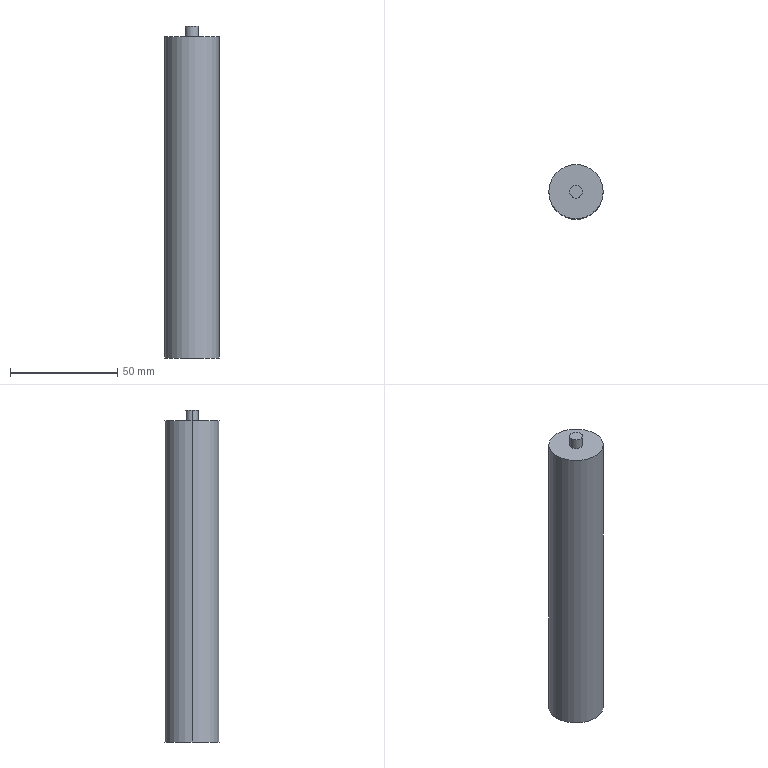Part | SolidWorks | features BaseBody 1 | 1 solid | 10 faces | box 25.4 x 25.4 x 155 mm | volume 75865 mm3 | cylinder 6 | plane 4 | commonest cylinder face diameters 6 x4 25.4 x2
STEP:
#1=CARTESIAN_POINT('',(12.7,0.,-150.));
#2=VERTEX_POINT('',#1);
#3=CARTESIAN_POINT('',(-12.7,0.,-150.));
#4=VERTEX_POINT('',#3);
#5=CARTESIAN_POINT('',(0.,0.,-150.));
#6=DIRECTION('',(0.,0.,1.));
#7=DIRECTION('',(1.,0.,0.));
#8=AXIS2_PLACEMENT_3D('',#5,#6,#7);
#9=CIRCLE('',#8,12.7);
#10=EDGE_CURVE('',#2,#4,#9,.T.);
#11=ORIENTED_EDGE('',*,*,#10,.T.);
#12=CARTESIAN_POINT('',(-12.7,0.,0.));
#13=VERTEX_POINT('',#12);
#14=CARTESIAN_POINT('',(-12.7,0.,-150.));
#15=DIRECTION('',(0.,0.,1.));
#16=VECTOR('',#15,1000.);
#17=LINE('',#14,#16);
#18=EDGE_CURVE('',#4,#13,#17,.T.);
#19=ORIENTED_EDGE('',*,*,#18,.T.);
#20=CARTESIAN_POINT('',(12.7,0.,0.));
#21=VERTEX_POINT('',#20);
#22=CARTESIAN_POINT('',(0.,0.,0.));
#23=DIRECTION('',(0.,0.,-1.));
#24=DIRECTION('',(1.,0.,0.));
#25=AXIS2_PLACEMENT_3D('',#22,#23,#24);
#26=CIRCLE('',#25,12.7);
#27=EDGE_CURVE('',#13,#21,#26,.T.);
#28=ORIENTED_EDGE('',*,*,#27,.T.);
#29=CARTESIAN_POINT('',(12.7,0.,-150.));
#30=DIRECTION('',(0.,0.,1.));
#31=VECTOR('',#30,1000.);
#32=LINE('',#29,#31);
#33=EDGE_CURVE('',#2,#21,#32,.T.);
#34=ORIENTED_EDGE('',*,*,#33,.F.);
#35=EDGE_LOOP('',(#11,#19,#28,#34));
#36=FACE_OUTER_BOUND('',#35,.T.);
#37=CARTESIAN_POINT('',(0.,0.,-150.));
#38=DIRECTION('',(0.,0.,1.));
#39=DIRECTION('',(1.,0.,0.));
#40=AXIS2_PLACEMENT_3D('',#37,#38,#39);
#41=CYLINDRICAL_SURFACE('',#40,12.7);
#42=ADVANCED_FACE('',(#36),#41,.T.);
#43=CARTESIAN_POINT('',(-3.,0.,5.));
#44=VERTEX_POINT('',#43);
#45=CARTESIAN_POINT('',(3.,0.,5.));
#46=VERTEX_POINT('',#45);
#47=CARTESIAN_POINT('',(0.,0.,5.));
#48=DIRECTION('',(0.,0.,-1.));
#49=DIRECTION('',(-1.,0.,0.));
#50=AXIS2_PLACEMENT_3D('',#47,#48,#49);
#51=CIRCLE('',#50,3.);
#52=EDGE_CURVE('',#44,#46,#51,.T.);
#53=ORIENTED_EDGE('',*,*,#52,.T.);
#54=CARTESIAN_POINT('',(3.,0.,0.));
#55=VERTEX_POINT('',#54);
#56=CARTESIAN_POINT('',(3.,0.,5.));
#57=DIRECTION('',(0.,0.,-1.));
#58=VECTOR('',#57,1000.);
#59=LINE('',#56,#58);
#60=EDGE_CURVE('',#46,#55,#59,.T.);
#61=ORIENTED_EDGE('',*,*,#60,.T.);
#62=CARTESIAN_POINT('',(-3.,0.,0.));
#63=VERTEX_POINT('',#62);
#64=CARTESIAN_POINT('',(0.,0.,0.));
#65=DIRECTION('',(0.,0.,-1.));
#66=DIRECTION('',(-1.,0.,0.));
#67=AXIS2_PLACEMENT_3D('',#64,#65,#66);
#68=CIRCLE('',#67,3.);
#69=EDGE_CURVE('',#63,#55,#68,.T.);
#70=ORIENTED_EDGE('',*,*,#69,.F.);
#71=CARTESIAN_POINT('',(-3.,0.,5.));
#72=DIRECTION('',(0.,0.,-1.));
#73=VECTOR('',#72,1000.);
#74=LINE('',#71,#73);
#75=EDGE_CURVE('',#44,#63,#74,.T.);
#76=ORIENTED_EDGE('',*,*,#75,.F.);
#77=EDGE_LOOP('',(#53,#61,#70,#76));
#78=FACE_OUTER_BOUND('',#77,.T.);
#79=CARTESIAN_POINT('',(0.,0.,5.));
#80=DIRECTION('',(0.,0.,-1.));
#81=DIRECTION('',(-1.,0.,0.));
#82=AXIS2_PLACEMENT_3D('',#79,#80,#81);
#83=CYLINDRICAL_SURFACE('',#82,3.);
#84=ADVANCED_FACE('',(#78),#83,.T.);
#85=CARTESIAN_POINT('',(3.,0.,-140.));
#86=VERTEX_POINT('',#85);
#87=CARTESIAN_POINT('',(-3.,0.,-140.));
#88=VERTEX_POINT('',#87);
#89=CARTESIAN_POINT('',(0.,0.,-140.));
#90=DIRECTION('',(0.,0.,-1.));
#91=DIRECTION('',(-1.,0.,0.));
#92=AXIS2_PLACEMENT_3D('',#89,#90,#91);
#93=CIRCLE('',#92,3.);
#94=EDGE_CURVE('',#86,#88,#93,.T.);
#95=ORIENTED_EDGE('',*,*,#94,.F.);
#96=CARTESIAN_POINT('',(3.,0.,-150.));
#97=VERTEX_POINT('',#96);
#98=CARTESIAN_POINT('',(3.,0.,-140.));
#99=DIRECTION('',(0.,0.,-1.));
#100=VECTOR('',#99,1000.);
#101=LINE('',#98,#100);
#102=EDGE_CURVE('',#86,#97,#101,.T.);
#103=ORIENTED_EDGE('',*,*,#102,.T.);
#104=CARTESIAN_POINT('',(-3.,0.,-150.));
#105=VERTEX_POINT('',#104);
#106=CARTESIAN_POINT('',(0.,0.,-150.));
#107=DIRECTION('',(0.,0.,-1.));
#108=DIRECTION('',(-1.,0.,0.));
#109=AXIS2_PLACEMENT_3D('',#106,#107,#108);
#110=CIRCLE('',#109,3.);
#111=EDGE_CURVE('',#97,#105,#110,.T.);
#112=ORIENTED_EDGE('',*,*,#111,.T.);
#113=CARTESIAN_POINT('',(-3.,0.,-140.));
#114=DIRECTION('',(0.,0.,-1.));
#115=VECTOR('',#114,1000.);
#116=LINE('',#113,#115);
#117=EDGE_CURVE('',#88,#105,#116,.T.);
#118=ORIENTED_EDGE('',*,*,#117,.F.);
#119=EDGE_LOOP('',(#95,#103,#112,#118));
#120=FACE_OUTER_BOUND('',#119,.T.);
#121=CARTESIAN_POINT('',(0.,0.,-140.));
#122=DIRECTION('',(0.,0.,-1.));
#123=DIRECTION('',(-1.,0.,0.));
#124=AXIS2_PLACEMENT_3D('',#121,#122,#123);
#125=CYLINDRICAL_SURFACE('',#124,3.);
#126=ADVANCED_FACE('',(#120),#125,.F.);
#127=ORIENTED_EDGE('',*,*,#18,.F.);
#128=CARTESIAN_POINT('',(0.,0.,-150.));
#129=DIRECTION('',(0.,0.,1.));
#130=DIRECTION('',(1.,0.,0.));
#131=AXIS2_PLACEMENT_3D('',#128,#129,#130);
#132=CIRCLE('',#131,12.7);
#133=EDGE_CURVE('',#4,#2,#132,.T.);
#134=ORIENTED_EDGE('',*,*,#133,.T.);
#135=ORIENTED_EDGE('',*,*,#33,.T.);
#136=CARTESIAN_POINT('',(0.,0.,0.));
#137=DIRECTION('',(0.,0.,-1.));
#138=DIRECTION('',(1.,0.,0.));
#139=AXIS2_PLACEMENT_3D('',#136,#137,#138);
#140=CIRCLE('',#139,12.7);
#141=EDGE_CURVE('',#21,#13,#140,.T.);
#142=ORIENTED_EDGE('',*,*,#141,.T.);
#143=EDGE_LOOP('',(#127,#134,#135,#142));
#144=FACE_OUTER_BOUND('',#143,.T.);
#145=CARTESIAN_POINT('',(0.,0.,-150.));
#146=DIRECTION('',(0.,0.,1.));
#147=DIRECTION('',(1.,0.,0.));
#148=AXIS2_PLACEMENT_3D('',#145,#146,#147);
#149=CYLINDRICAL_SURFACE('',#148,12.7);
#150=ADVANCED_FACE('',(#144),#149,.T.);
#151=ORIENTED_EDGE('',*,*,#141,.F.);
#152=ORIENTED_EDGE('',*,*,#27,.F.);
#153=EDGE_LOOP('',(#151,#152));
#154=FACE_OUTER_BOUND('',#153,.T.);
#155=ORIENTED_EDGE('',*,*,#69,.T.);
#156=CARTESIAN_POINT('',(0.,0.,0.));
#157=DIRECTION('',(0.,0.,-1.));
#158=DIRECTION('',(-1.,0.,0.));
#159=AXIS2_PLACEMENT_3D('',#156,#157,#158);
#160=CIRCLE('',#159,3.);
#161=EDGE_CURVE('',#55,#63,#160,.T.);
#162=ORIENTED_EDGE('',*,*,#161,.T.);
#163=EDGE_LOOP('',(#155,#162));
#164=FACE_BOUND('',#163,.T.);
#165=CARTESIAN_POINT('',(0.,0.,0.));
#166=DIRECTION('',(0.,0.,1.));
#167=DIRECTION('',(1.,0.,0.));
#168=AXIS2_PLACEMENT_3D('',#165,#166,#167);
#169=PLANE('',#168);
#170=ADVANCED_FACE('',(#154,#164),#169,.T.);
#171=ORIENTED_EDGE('',*,*,#10,.F.);
#172=ORIENTED_EDGE('',*,*,#133,.F.);
#173=EDGE_LOOP('',(#171,#172));
#174=FACE_OUTER_BOUND('',#173,.T.);
#175=CARTESIAN_POINT('',(0.,0.,-150.));
#176=DIRECTION('',(0.,0.,-1.));
#177=DIRECTION('',(-1.,0.,0.));
#178=AXIS2_PLACEMENT_3D('',#175,#176,#177);
#179=CIRCLE('',#178,3.);
#180=EDGE_CURVE('',#105,#97,#179,.T.);
#181=ORIENTED_EDGE('',*,*,#180,.F.);
#182=ORIENTED_EDGE('',*,*,#111,.F.);
#183=EDGE_LOOP('',(#181,#182));
#184=FACE_BOUND('',#183,.T.);
#185=CARTESIAN_POINT('',(0.,0.,-150.));
#186=DIRECTION('',(0.,0.,1.));
#187=DIRECTION('',(1.,0.,0.));
#188=AXIS2_PLACEMENT_3D('',#185,#186,#187);
#189=PLANE('',#188);
#190=ADVANCED_FACE('',(#174,#184),#189,.F.);
#191=ORIENTED_EDGE('',*,*,#60,.F.);
#192=CARTESIAN_POINT('',(0.,0.,5.));
#193=DIRECTION('',(0.,0.,-1.));
#194=DIRECTION('',(-1.,0.,0.));
#195=AXIS2_PLACEMENT_3D('',#192,#193,#194);
#196=CIRCLE('',#195,3.);
#197=EDGE_CURVE('',#46,#44,#196,.T.);
#198=ORIENTED_EDGE('',*,*,#197,.T.);
#199=ORIENTED_EDGE('',*,*,#75,.T.);
#200=ORIENTED_EDGE('',*,*,#161,.F.);
#201=EDGE_LOOP('',(#191,#198,#199,#200));
#202=FACE_OUTER_BOUND('',#201,.T.);
#203=CARTESIAN_POINT('',(0.,0.,5.));
#204=DIRECTION('',(0.,0.,-1.));
#205=DIRECTION('',(-1.,0.,0.));
#206=AXIS2_PLACEMENT_3D('',#203,#204,#205);
#207=CYLINDRICAL_SURFACE('',#206,3.);
#208=ADVANCED_FACE('',(#202),#207,.T.);
#209=ORIENTED_EDGE('',*,*,#102,.F.);
#210=CARTESIAN_POINT('',(0.,0.,-140.));
#211=DIRECTION('',(0.,0.,-1.));
#212=DIRECTION('',(-1.,0.,0.));
#213=AXIS2_PLACEMENT_3D('',#210,#211,#212);
#214=CIRCLE('',#213,3.);
#215=EDGE_CURVE('',#88,#86,#214,.T.);
#216=ORIENTED_EDGE('',*,*,#215,.F.);
#217=ORIENTED_EDGE('',*,*,#117,.T.);
#218=ORIENTED_EDGE('',*,*,#180,.T.);
#219=EDGE_LOOP('',(#209,#216,#217,#218));
#220=FACE_OUTER_BOUND('',#219,.T.);
#221=CARTESIAN_POINT('',(0.,0.,-140.));
#222=DIRECTION('',(0.,0.,-1.));
#223=DIRECTION('',(-1.,0.,0.));
#224=AXIS2_PLACEMENT_3D('',#221,#222,#223);
#225=CYLINDRICAL_SURFACE('',#224,3.);
#226=ADVANCED_FACE('',(#220),#225,.F.);
#227=ORIENTED_EDGE('',*,*,#52,.F.);
#228=ORIENTED_EDGE('',*,*,#197,.F.);
#229=EDGE_LOOP('',(#227,#228));
#230=FACE_OUTER_BOUND('',#229,.T.);
#231=CARTESIAN_POINT('',(0.,0.,5.));
#232=DIRECTION('',(0.,0.,1.));
#233=DIRECTION('',(1.,0.,0.));
#234=AXIS2_PLACEMENT_3D('',#231,#232,#233);
#235=PLANE('',#234);
#236=ADVANCED_FACE('',(#230),#235,.T.);
#237=ORIENTED_EDGE('',*,*,#215,.T.);
#238=ORIENTED_EDGE('',*,*,#94,.T.);
#239=EDGE_LOOP('',(#237,#238));
#240=FACE_OUTER_BOUND('',#239,.T.);
#241=CARTESIAN_POINT('',(0.,0.,-140.));
#242=DIRECTION('',(0.,0.,-1.));
#243=DIRECTION('',(-1.,0.,0.));
#244=AXIS2_PLACEMENT_3D('',#241,#242,#243);
#245=PLANE('',#244);
#246=ADVANCED_FACE('',(#240),#245,.T.);
#247=CLOSED_SHELL('',(#42,#84,#126,#150,#170,#190,#208,#226,#236,#246));
#248=MANIFOLD_SOLID_BREP('',#247);
#249=CARTESIAN_POINT('',(0.,0.,0.));
#250=DIRECTION('',(0.,0.,1.));
#251=DIRECTION('',(1.,0.,0.));
#252=AXIS2_PLACEMENT_3D('',#249,#250,#251);
#253=(LENGTH_UNIT()NAMED_UNIT(*)SI_UNIT(.MILLI.,.METRE.));
#254=UNCERTAINTY_MEASURE_WITH_UNIT(LENGTH_MEASURE(0.00001),#253,'','');
#255=(NAMED_UNIT(*)PLANE_ANGLE_UNIT()SI_UNIT($,.RADIAN.));
#256=(NAMED_UNIT(*)SI_UNIT($,.STERADIAN.)SOLID_ANGLE_UNIT());
#257=(GEOMETRIC_REPRESENTATION_CONTEXT(3)GLOBAL_UNCERTAINTY_ASSIGNED_CONTEXT((#254))GLOBAL_UNIT_ASSIGNED_CONTEXT((#253,#255,#256))REPRESENTATION_CONTEXT('',''));
#258=ADVANCED_BREP_SHAPE_REPRESENTATION('',(#248,#252),#257);